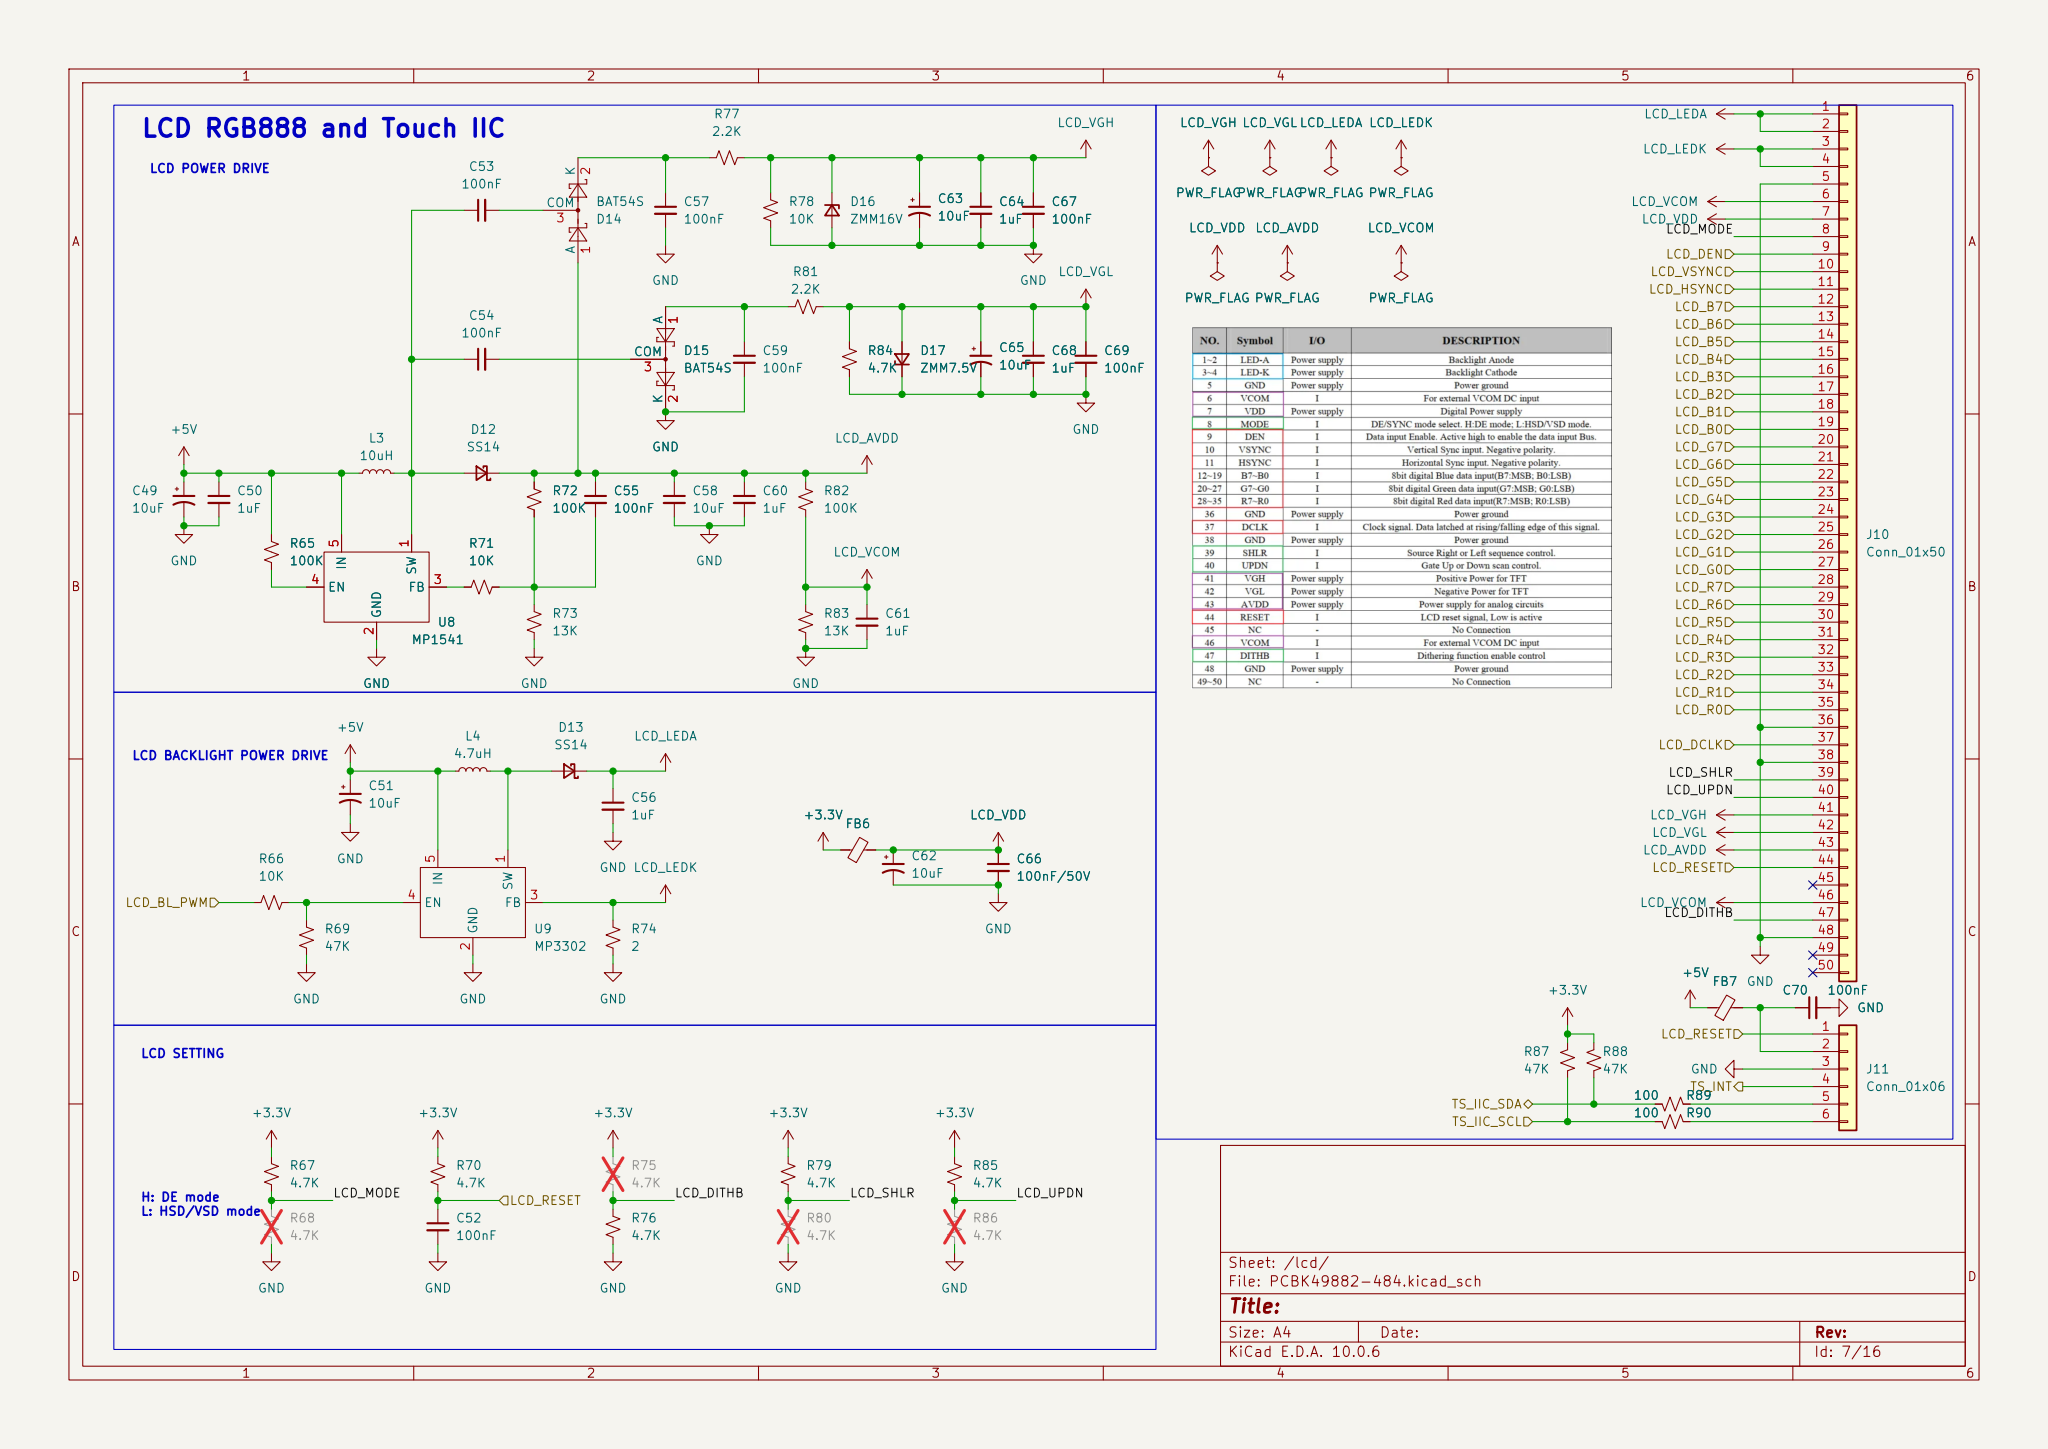Circuit board | KiCad | 536 parts | 438 nets | one sheet of the schematic
Parts on this sheet (reference | value | footprint):
C49 | 10uF | Capacitor_Tantalum_SMD:CP_EIA-3216-18_Kemet-A
C50 | 1uF | Capacitor_SMD:C_0603_1608Metric
C51 | 10uF | Capacitor_Tantalum_SMD:CP_EIA-3216-18_Kemet-A
C52
C53
C54
C55
C56 | 1uF | Capacitor_SMD:C_1210_3225Metric
C57 | 100nF | Capacitor_SMD:C_0603_1608Metric
C58 | 10uF | Capacitor_SMD:C_1210_3225Metric
C59 | 100nF | Capacitor_SMD:C_0603_1608Metric
C60 | 1uF | Capacitor_SMD:C_0603_1608Metric
C61 | 1uF | Capacitor_SMD:C_0603_1608Metric
C62 | 10uF | Capacitor_Tantalum_SMD:CP_EIA-3216-18_Kemet-A
C63 | 10uF | Capacitor_Tantalum_SMD:CP_EIA-3216-18_Kemet-A
C64 | 1uF | Capacitor_SMD:C_1210_3225Metric
C65 | 10uF | Capacitor_Tantalum_SMD:CP_EIA-3216-18_Kemet-A
C66 | 100nF/50V | Capacitor_SMD:C_0603_1608Metric
C67 | 100nF | Capacitor_SMD:C_0603_1608Metric
C68 | 1uF | Capacitor_SMD:C_1210_3225Metric
C69
C70
D12 | SS14 | Diode_SMD:D_SMA
D13 | SS14 | Diode_SMD:D_SMA
D14 | BAT54S | Package_TO_SOT_SMD:SOT-23
D15 | BAT54S | Package_TO_SOT_SMD:SOT-23
D16 | ZMM16V | Diode_SMD:D_1206_3216Metric
D17 | ZMM7.5V | Diode_SMD:D_1206_3216Metric
FB6 | 100ohm @100MHz max. 4000mA | Inductor_SMD:L_0805_2012Metric
FB7 | 100ohm @100MHz max. 4000mA | Inductor_SMD:L_0603_1608Metric
J10 | Conn_01x50 | Connector_FFC-FPC:Hirose_FH12-50S-0.5SH_1x50-1MP_P0.50mm_Horizontal
J11 | Conn_01x06 | Connector_FFC-FPC:Hirose_FH12-6S-0.5SH_1x06-1MP_P0.50mm_Horizontal
L3 | 10uH | Inductor_SMD:L_Changjiang_FNR4030S
L4 | 4.7uH | Inductor_SMD:L_Changjiang_FNR4030S
R65 | 100K | Resistor_SMD:R_0603_1608Metric
R66 | 10K | Resistor_SMD:R_0603_1608Metric
R67 | 4.7K | Resistor_SMD:R_0603_1608Metric
R68 | 4.7K | Resistor_SMD:R_0603_1608Metric
R69 | 47K | Resistor_SMD:R_0603_1608Metric
R71 | 10K | Resistor_SMD:R_0603_1608Metric
R72 | 100K | Resistor_SMD:R_0603_1608Metric
R73 | 13K | Resistor_SMD:R_0603_1608Metric
R74 | 2 | Resistor_SMD:R_0603_1608Metric
R75 | 4.7K | Resistor_SMD:R_0603_1608Metric
R76 | 4.7K | Resistor_SMD:R_0603_1608Metric
R78 | 10K | Resistor_SMD:R_0603_1608Metric
R79 | 4.7K | Resistor_SMD:R_0603_1608Metric
R80 | 4.7K | Resistor_SMD:R_0603_1608Metric
R81 | 2.2K | Resistor_SMD:R_0603_1608Metric
R82 | 100K | Resistor_SMD:R_0603_1608Metric
R83 | 13K | Resistor_SMD:R_0603_1608Metric
R84
R85
R86
R87 | 47K | Resistor_SMD:R_0603_1608Metric
R88 | 47K | Resistor_SMD:R_0603_1608Metric
R89 | 100 | Resistor_SMD:R_0603_1608Metric
R90 | 100 | Resistor_SMD:R_0603_1608Metric
U8 | MP1541 | Package_TO_SOT_SMD:SOT-23-5
Nets of these parts (net: part-pin ...):
+3.3V: FB6-1 R67-2 R75-2 R79-2 R85-2 R87-2 R88-2
+5V: C49-1 C50-1 C51-1 FB7-1 L3-1 L4-1 R65-2 U8-5
/core_board_b2b/NRST: C52-1 J11-1 J10-44
/core_board_b2b/PA8{slash}LCD_BL_PWM: R66-1
/core_board_b2b/PH4{slash}IIC2_SCL: R87-1 R90-2
/core_board_b2b/PH5{slash}IIC2_SDA: R88-1 R89-2
/core_board_b2b/PH7{slash}TS_INT: J11-4
/lcd/LCD_DITHB: R75-1 R76-2 J10-47
/lcd/LCD_MODE: R67-1 R68-2 J10-8
/lcd/LCD_SHLR: R79-1 R80-2 J10-39
/lcd/LCD_UPDN: R85-1 R86-2 J10-40
GND: C49-2 C50-2 C51-2 C52-2 C56-2 C57-2 C58-2 C59-2 C60-2 C61-2 C62-2 C63-2 C64-2 C65-2 C66-2 C67-2 C68-2 C69-2 C70-2 D15-2 D16-2 D17-1 J11-3 R68-1 R69-1 R73-1 R74-1 R76-1 R78-1 R80-1 R83-1 R84-1 R86-1 U8-2 J10-5 J10-36 J10-38 J10-48
LCD_AVDD: C55-1 C58-1 C60-1 D12-1 D14-1 R72-2 R82-2 J10-43
LCD_LEDA: C56-1 D13-1 J10-1 J10-2
LCD_LEDK: R74-2 J10-3 J10-4
LCD_VCOM: C61-1 R82-1 R83-2 J10-6 J10-46
LCD_VDD: C62-1 C66-1 FB6-2 J10-7
LCD_VGH: C63-1 C64-1 C67-1 D16-1 R78-2 J10-41
LCD_VGL: C65-1 C68-1 C69-1 D17-2 R81-2 R84-2 J10-42
Net-(C55-Pad2): C55-2 R71-2 R72-1 R73-2
Net-(D12-A): C53-1 C54-1 D12-2 L3-2 U8-1
Net-(D13-A): D13-2 L4-2
Net-(D14-COM): C53-2 D14-3
Net-(D14-K): C57-1 D14-2
Net-(D15-A): C59-1 D15-1 R81-1
Net-(D15-COM): C54-2 D15-3
Net-(J11-Pin_2): C70-1 FB7-2 J11-2
Net-(J11-Pin_5): J11-5 R89-1
Net-(J11-Pin_6): J11-6 R90-1
Net-(U8-EN): R65-1 U8-4
Net-(U8-FB): R71-1 U8-3
Net-(U9-EN): R66-2 R69-2